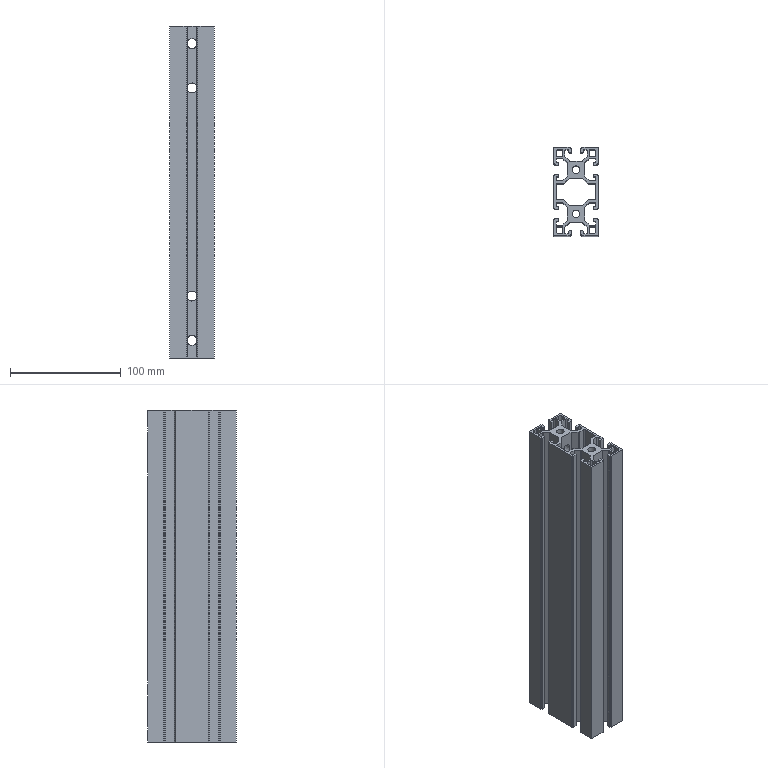Part | SolidWorks | features 3DProfileFeature 2, HoleWzd 2, Extrusion 1 | 1 solid | 444 faces | box 40 x 80 x 300 mm | volume 325543 mm3 | cylinder 254 | plane 190 | commonest cylinder face diameters 0.6 x126 2 x40 9 x24 0.4 x20 6.8 x20 15 x16